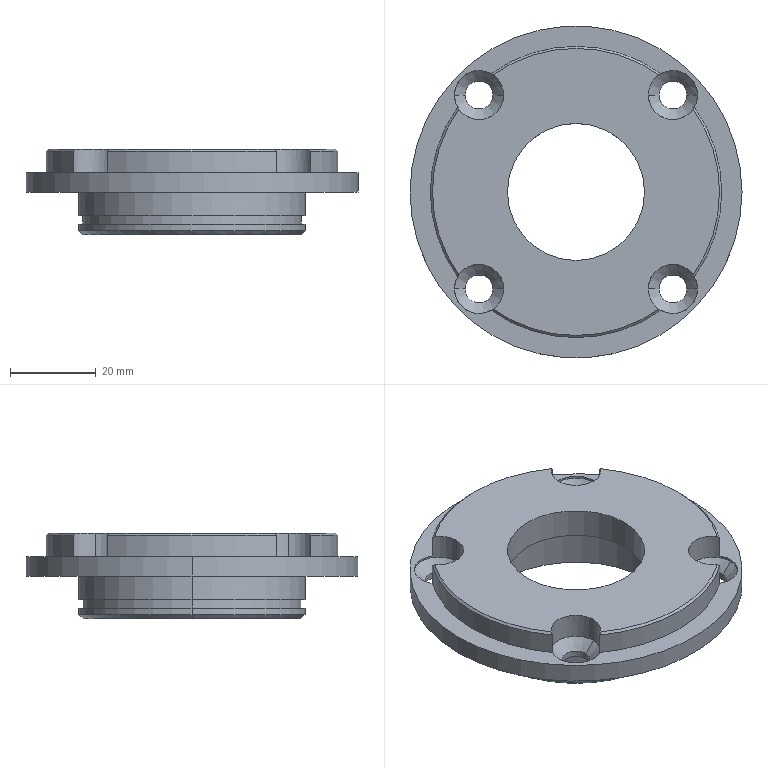Part | SolidWorks | features BaseBody 1 | 1 solid | 57 faces | box 77.5 x 77.5 x 20 mm | volume 32687 mm3 | cylinder 35 | cone 14 | plane 8 | commonest cylinder face diameters 6.5 x8 11.5 x8 68 x5 53 x4 32 x2 42 x2